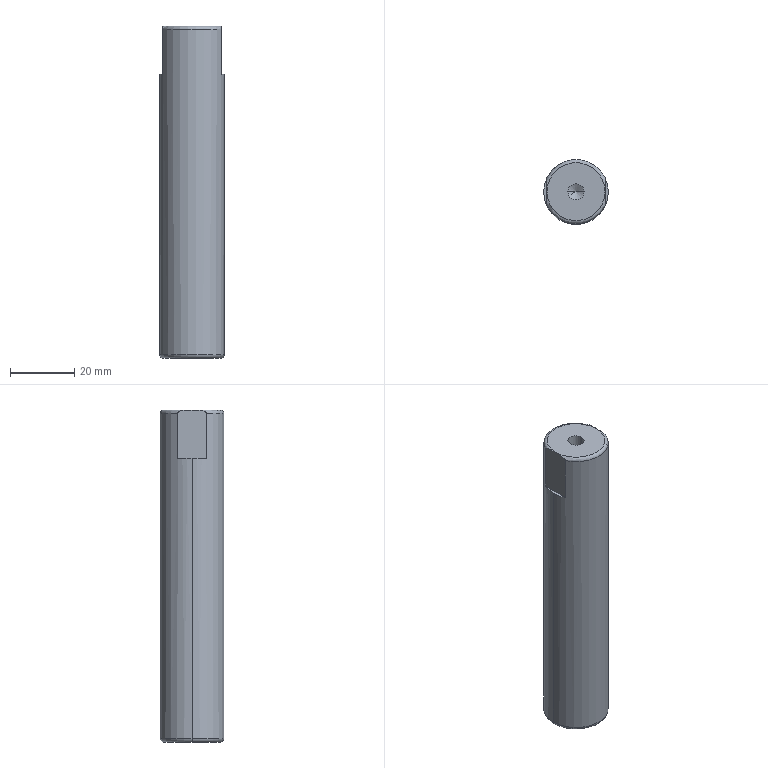Part | STEP file | 1 solid | 20 faces | box 20 x 20 x 103 mm | volume 31531 mm3 | cylinder 6 | plane 6 | torus 4 | cone 4 | commonest cylinder face diameters 5 x4 20 x2